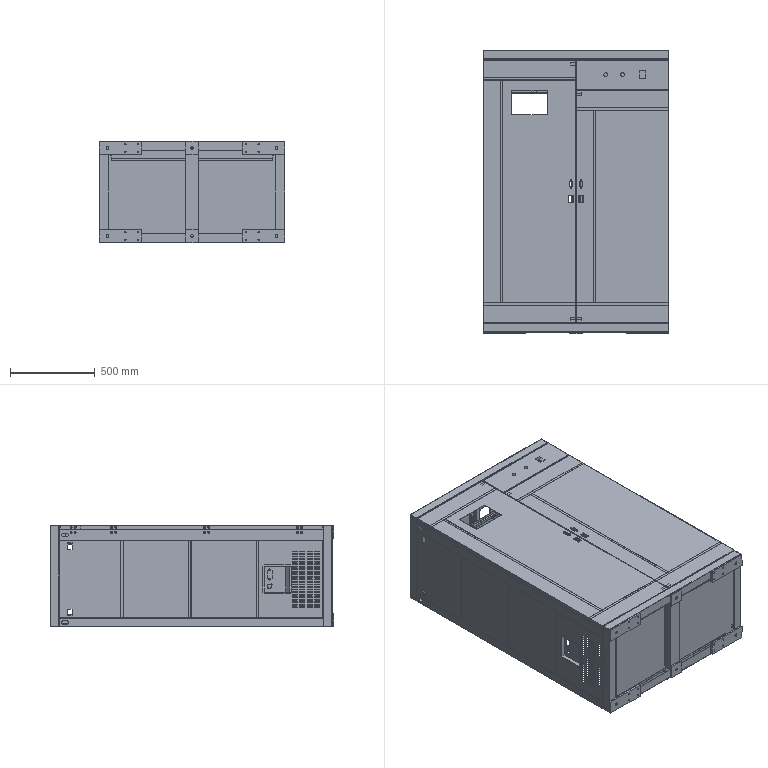Part | SolidWorks | features ICE 63, FlatPattern 34, SMBaseFlange 34, SheetMetal 34, LPattern 21, MirrorSolid 19, EdgeFlange 14, BossThin 9, MirrorPattern 6, SMMiteredFlange 6, Chamfer 2, CornerTrim 1, Split 1 | 73 solids | 4367 faces | volume 13322104 mm3 | plane 2300 | cylinder 1913 | spline 154 | commonest cylinder face diameters 5 x368 4.5 x360 5.5 x296 0.2 x190 10.5 x162 3.2 x103